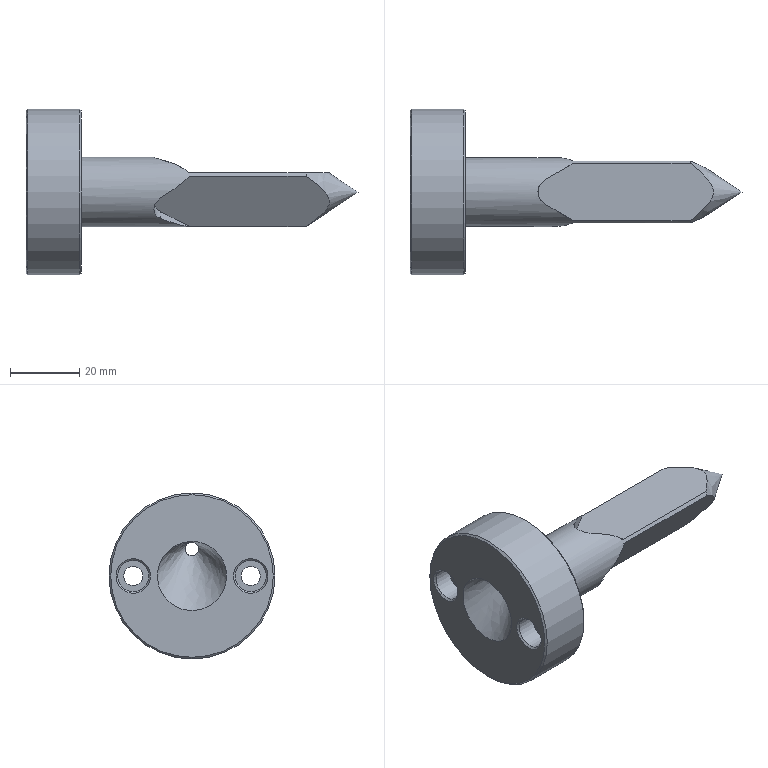NC program | NX | posted with a generic post | part box 96 x 48 x 48 mm
Lines 1 to 1795 of 1974, first 1661 of 1787 lines:
N10 G17 G21 G94 G90
(FLOOR_WALL , TOOL : D8)
N12 T08 M6
N14 G54
N16 G17 G0 G90 X-66.284 Y-8.048 S3500 M3
N18 G43 Z34.062 H8
N20 Z9.788
N22 G94 G1 X-69.517 Y-2.448 F1001.
N24 G3 X-70.21 Y-2.048 R0.8
N26 G1 X-95.937 F2200.
N28 Y2.048
N30 X-44.483
N32 X-41.035 Y0.
N34 X-44.482 Y-2.048
N36 X-70.21
N38 G3 X-70.903 Y-2.448 R0.8
N40 G1 X-74.136 Y-8.048
N42 G0 X-66.984 Y-8.881 Z9.576
N44 G1 X-70.218 Y-3.281 F1001.
N46 G3 X-70.91 Y-2.881 R0.8
N48 G1 X-95.937 F2200.
N50 Y2.881
N52 X-45.884
N54 X-41.035 Y0.
N56 X-45.883 Y-2.881
N58 X-70.91
N60 G3 X-71.603 Y-3.281 R0.8
N62 G1 X-74.836 Y-8.881
N64 G0 X-67.513 Y-9.509 Z9.364
N66 G1 X-70.746 Y-3.909 F1001.
N68 G3 X-71.439 Y-3.509 R0.8
N70 G1 X-95.937 F2200.
N72 Y3.509
N74 X-46.941
N76 X-41.035 Y0.
N78 X-46.941 Y-3.509
N80 X-71.439
N82 G3 X-72.132 Y-3.909 R0.8
N84 G1 X-75.365 Y-9.509
N86 G0 X-66.5 Y-10.029 Z9.152
N88 G1 X-69.733 Y-4.429 F1001.
N90 G3 X-70.426 Y-4.029 R0.8
N92 G1 X-95.937 F2200.
N94 Y4.029
N96 X-47.817
N98 X-41.035 Y0.
N100 X-47.817 Y-4.029
N102 X-70.426
N104 Y-0.029
N106 X-91.937
N108 Y0.029
N110 X-48.916
N112 X-48.866 Y0.
N114 X-48.915 Y-0.029
N116 X-70.426
N118 G3 X-71.119 Y-0.429 R0.8
N120 G1 Y-10.029
N122 G0 X-66.879 Y-10.48 Z8.94
N124 G1 X-70.113 Y-4.88 F1001.
N126 G3 X-70.805 Y-4.48 R0.8
N128 G1 X-95.937 F2200.
N130 Y4.48
N132 X-48.575
N134 X-41.035 Y0.
N136 X-48.575 Y-4.48
N138 X-70.805
N140 Y-0.48
N142 X-91.937
N144 Y0.48
N146 X-49.674
N148 X-48.866 Y0.
N150 X-49.674 Y-0.48
N152 X-70.805
N154 G3 X-71.498 Y-0.88 R0.8
N156 G1 Y-10.48
N158 G0 X-67.216 Y-10.88 Z8.729
N160 G1 X-70.449 Y-5.28 F1001.
N162 G3 X-71.142 Y-4.88 R0.8
N164 G1 X-95.92 F2200.
N166 X-95.937 Y-4.869
N168 Y4.869
N170 X-95.92 Y4.88
N172 X-49.249
N174 X-41.035 Y0.
N176 X-49.248 Y-4.88
N178 X-71.142
N180 Y-0.88
N182 X-91.937
N184 Y0.88
N186 X-50.347
N188 X-48.866 Y0.
N190 X-50.347 Y-0.88
N192 X-71.142
N194 G3 X-71.835 Y-1.28 R0.8
N196 G1 Y-10.88
N198 G0 X-67.52 Y-11.241 Z8.517
N200 G1 X-70.753 Y-5.641 F1001.
N202 G3 X-71.446 Y-5.241 R0.8
N204 G1 X-95.379 F2200.
N206 X-95.937 Y-4.869
N208 Y4.869
N210 X-95.379 Y5.241
N212 X-49.856
N214 X-41.035 Y0.
N216 X-49.856 Y-5.241
N218 X-71.446
N220 Y-1.241
N222 X-91.937
N224 Y1.241
N226 X-50.955
N228 X-48.866 Y0.
N230 X-50.955 Y-1.241
N232 X-71.446
N234 G3 X-72.139 Y-1.641 R0.8
N236 G1 Y-11.241
N238 G0 X-67.797 Y-11.571 Z8.305
N240 G1 X-71.031 Y-5.971 F1001.
N242 G3 X-71.723 Y-5.571 R0.8
N244 G1 X-94.884 F2200.
N246 X-95.937 Y-4.869
N248 Y4.869
N250 X-94.884 Y5.571
N252 X-50.411
N254 X-41.035 Y0.
N256 X-50.411 Y-5.571
N258 X-71.723
N260 Y-1.571
N262 X-91.937
N264 Y1.571
N266 X-51.51
N268 X-48.866 Y0.
N270 X-51.51 Y-1.571
N272 X-71.723
N274 G3 X-72.416 Y-1.971 R0.8
N276 G1 Y-11.571
N278 G0 X-68.053 Y-11.874 Z8.093
N280 G1 X-71.286 Y-6.274 F1001.
N282 G3 X-71.979 Y-5.874 R0.8
N284 G1 X-94.429 F2200.
N286 X-95.937 Y-4.869
N288 Y4.869
N290 X-94.429 Y5.874
N292 X-50.922
N294 X-41.035 Y0.
N296 X-50.922 Y-5.874
N298 X-71.979
N300 Y-1.874
N302 X-91.937
N304 Y1.874
N306 X-52.021
N308 X-48.866 Y0.
N310 X-52.021 Y-1.874
N312 X-71.979
N314 G3 X-72.672 Y-2.274 R0.8
N316 G1 Y-11.874
N318 G0 X-68.29 Y-12.156 Z7.881
N320 G1 X-71.523 Y-6.556 F1001.
N322 G3 X-72.216 Y-6.156 R0.8
N324 G1 X-94.007 F2200.
N326 X-95.937 Y-4.869
N328 Y4.869
N330 X-94.007 Y6.156
N332 X-51.396
N334 X-41.035 Y0.
N336 X-51.396 Y-6.156
N338 X-72.216
N340 Y-2.156
N342 X-91.937
N344 Y2.156
N346 X-52.494
N348 X-48.866 Y0.
N350 X-52.494 Y-2.156
N352 X-72.216
N354 G3 X-72.909 Y-2.556 R0.8
N356 G1 Y-12.156
N358 G0 X-68.51 Y-12.418 Z7.669
N360 G1 X-71.743 Y-6.818 F1001.
N362 G3 X-72.436 Y-6.418 R0.8
N364 G1 X-93.614 F2200.
N366 X-95.937 Y-4.869
N368 Y4.869
N370 X-93.614 Y6.418
N372 X-51.829
N374 X-41.035 Y0.
N376 X-51.829 Y-6.418
N378 X-72.436
N380 Y-2.418
N382 X-91.937
N384 Y2.418
N386 X-52.936
N388 X-48.866 Y0.
N390 X-52.935 Y-2.418
N392 X-72.436
N394 G3 X-73.129 Y-2.818 R0.8
N396 G1 Y-12.418
N398 G0 X-68.716 Y-12.663 Z7.457
N400 G1 X-71.95 Y-7.063 F1001.
N402 G3 X-72.642 Y-6.663 R0.8
N404 G1 X-93.246 F2200.
N406 X-95.937 Y-4.869
N408 Y4.869
N410 X-93.246 Y6.663
N412 X-51.762
N414 X-51.83 Y6.414
N416 X-41.035 Y0.
N418 X-51.83 Y-6.414
N420 X-51.762 Y-6.663
N422 X-72.642
N424 Y-2.663
N426 X-91.937
N428 Y2.663
N430 X-53.348
N432 X-48.866 Y0.
N434 X-53.348 Y-2.663
N436 X-72.642
N438 G3 X-73.335 Y-3.063 R0.8
N440 G1 Y-12.663
N442 G0 X-68.786 Y-12.892 Z7.245
N444 G1 X-72.02 Y-7.292 F1001.
N446 G3 X-72.712 Y-6.892 R0.8
N448 G1 X-92.901 F2200.
N450 X-95.937 Y-4.869
N452 Y4.869
N454 X-92.901 Y6.893
N456 X-51.699
N458 X-51.83 Y6.414
N460 X-41.035 Y0.
N462 X-51.83 Y-6.414
N464 X-51.699 Y-6.892
N466 X-72.712
N468 Y-2.892
N470 X-91.69
N472 X-91.937 Y-2.728
N474 Y2.728
N476 X-91.69 Y2.893
N478 X-53.735
N480 X-48.866 Y0.
N482 X-53.734 Y-2.892
N484 X-72.712
N486 G3 X-73.405 Y-3.292 R0.8
N488 G1 Y-12.892
N490 G0 X-68.799 Y-13.109 Z7.033
N492 G1 X-72.032 Y-7.509 F1001.
N494 G3 X-72.725 Y-7.109 R0.8
N496 G1 X-92.577 F2200.
N498 X-95.937 Y-4.869
N500 Y4.869
N502 X-92.577 Y7.109
N504 X-51.64
N506 X-51.83 Y6.414
N508 X-41.035 Y0.
N510 X-51.83 Y-6.414
N512 X-51.639 Y-7.109
N514 X-72.725
N516 Y-3.109
N518 X-91.366
N520 X-91.937 Y-2.728
N522 Y2.728
N524 X-91.366 Y3.109
N526 X-54.083
N528 G3 X-53.874 Y2.975 R4.
N530 G1 X-48.866 Y0.
N532 X-53.873 Y-2.975
N534 G3 X-54.083 Y-3.109 R4.
N536 G1 X-72.725
N538 G3 X-73.417 Y-3.509 R0.8
N540 G1 Y-13.109
N542 G0 X-68.782 Y-13.312 Z6.821
N544 G1 X-72.016 Y-7.712 F1001.
N546 G3 X-72.708 Y-7.312 R0.8
N548 G1 X-92.272 F2200.
N550 X-95.937 Y-4.869
N552 Y4.869
N554 X-92.272 Y7.312
N556 X-51.584
N558 X-51.83 Y6.414
N560 X-41.035 Y0.
N562 X-51.83 Y-6.414
N564 X-51.583 Y-7.312
N566 X-72.708
N568 Y-3.312
N570 X-91.061
N572 X-91.937 Y-2.728
N574 Y2.728
N576 X-91.061 Y3.312
N578 X-54.356
N580 G3 X-53.874 Y2.975 R4.
N582 G1 X-48.866 Y0.
N584 X-53.873 Y-2.975
N586 G3 X-54.356 Y-3.312 R4.
N588 G1 X-72.708
N590 G3 X-73.401 Y-3.712 R0.8
N592 G1 Y-13.312
N594 G0 X-68.748 Y-13.504 Z6.61
N596 G1 X-71.981 Y-7.904 F1001.
N598 G3 X-72.674 Y-7.504 R0.8
N600 G1 X-91.984 F2200.
N602 X-95.937 Y-4.869
N604 Y4.869
N606 X-91.983 Y7.504
N608 X-51.531
N610 X-51.83 Y6.414
N612 X-41.035 Y0.
N614 X-51.83 Y-6.414
N616 X-51.531 Y-7.504
N618 X-72.674
N620 Y-3.504
N622 X-90.773
N624 X-91.937 Y-2.728
N626 Y2.728
N628 X-90.772 Y3.504
N630 X-54.575
N632 G3 X-53.874 Y2.975 R4.
N634 G1 X-48.866 Y0.
N636 X-53.873 Y-2.975
N638 G3 X-54.575 Y-3.504 R4.
N640 G1 X-72.674
N642 G3 X-73.367 Y-3.904 R0.8
N644 G1 Y-13.504
N646 G0 X-68.262 Y-13.686 Z6.398
N648 G1 X-71.495 Y-8.086 F1001.
N650 G3 X-72.188 Y-7.686 R0.8
N652 G1 X-91.711 F2200.
N654 X-95.937 Y-4.869
N656 Y4.869
N658 X-91.711 Y7.686
N660 X-51.481
N662 X-51.83 Y6.414
N664 X-41.035 Y0.
N666 X-51.83 Y-6.414
N668 X-51.481 Y-7.686
N670 X-72.188
N672 Y-3.686
N674 X-90.5
N676 X-91.937 Y-2.728
N678 Y2.728
N680 X-90.5 Y3.686
N682 X-54.756
N684 G3 X-53.874 Y2.975 R4.
N686 G1 X-48.866 Y0.
N688 X-53.873 Y-2.975
N690 G3 X-54.755 Y-3.686 R4.
N692 G1 X-72.188
N694 Y-0.086
N696 X-88.337
N698 Y0.086
N700 X-56.039
N702 X-55.907 Y0.
N704 X-56.039 Y-0.086
N706 X-72.188
N708 G3 X-72.881 Y-0.486 R0.8
N710 G0 Z34.997
N712 X-72.382 Y-2.014 Z34.942
N714 X-71.882 Y-3.538 Z34.821
N716 X-71.383 Y-5.055 Z34.633
N718 X-70.883 Y-6.563 Z34.379
N720 X-70.384 Y-8.058 Z34.06
N722 X-69.884 Y-9.538 Z33.675
N724 X-69.385 Y-11. Z33.227
N726 X-68.885 Y-12.44 Z32.714
N728 X-68.386 Y-13.857 Z32.14
N730 Z6.186
N732 G1 X-71.619 Y-8.257 F1001.
N734 G3 X-72.312 Y-7.857 R0.8
N736 G1 X-91.454 F2200.
N738 X-95.937 Y-4.869
N740 Y4.869
N742 X-91.454 Y7.857
N744 X-51.434
N746 X-51.83 Y6.414
N748 X-41.035 Y0.
N750 X-51.83 Y-6.414
N752 X-51.434 Y-7.857
N754 X-72.312
N756 Y-3.857
N758 X-90.243
N760 X-91.937 Y-2.728
N762 Y2.728
N764 X-90.243 Y3.857
N766 X-54.907
N768 G3 X-53.874 Y2.975 R4.
N770 G1 X-48.866 Y0.
N772 X-53.873 Y-2.975
N774 G3 X-54.907 Y-3.857 R4.
N776 G1 X-72.312
N778 Y-0.257
N780 X-88.337
N782 Y0.257
N784 X-56.287
N786 G3 X-55.907 Y0. R7.6
N788 X-56.286 Y-0.257 R7.6
N790 G1 X-72.312
N792 G3 X-73.005 Y-0.657 R0.8
N794 G0 Z34.994
N796 X-72.489 Y-2.186 Z34.932
N798 X-71.973 Y-3.71 Z34.803
N800 X-71.457 Y-5.227 Z34.608
N802 X-70.941 Y-6.734 Z34.346
N804 X-70.425 Y-8.228 Z34.019
N806 X-69.909 Y-9.706 Z33.627
N808 X-69.393 Y-11.166 Z33.171
N810 X-68.877 Y-12.605 Z32.651
N812 X-68.362 Y-14.02 Z32.069
N814 Z5.974
N816 G1 X-71.595 Y-8.42 F1001.
N818 G3 X-72.288 Y-8.02 R0.8
N820 G1 X-91.211 F2200.
N822 X-95.937 Y-4.869
N824 Y4.869
N826 X-91.211 Y8.02
N828 X-51.389
N830 X-51.83 Y6.414
N832 X-41.035 Y0.
N834 X-51.83 Y-6.414
N836 X-51.389 Y-8.02
N838 X-72.288
N840 Y-4.02
N842 X-90.
N844 X-91.937 Y-2.728
N846 Y2.728
N848 X-89.999 Y4.02
N850 X-55.035
N852 G3 X-53.874 Y2.975 R4.
N854 G1 X-48.866 Y0.
N856 X-53.873 Y-2.975
N858 G3 X-55.034 Y-4.02 R4.
N860 G1 X-72.288
N862 Y-0.02
N864 X-87.937
N866 Y0.02
N868 X-56.638
N870 X-56.612 Y0.
N872 X-56.638 Y-0.02
N874 X-72.288
N876 G3 X-72.98 Y-0.42 R0.8
N878 G0 Z34.997
N880 X-72.478 Y-1.993 Z34.943
N882 X-71.976 Y-3.563 Z34.818
N884 X-71.474 Y-5.125 Z34.623
N886 X-70.971 Y-6.677 Z34.357
N888 X-70.469 Y-8.216 Z34.022
N890 X-69.967 Y-9.738 Z33.618
N892 X-69.465 Y-11.24 Z33.146
N894 X-68.963 Y-12.719 Z32.607
N896 X-68.46 Y-14.173 Z32.002
N898 Z5.762
N900 G1 X-71.694 Y-8.573 F1001.
N902 G3 X-72.386 Y-8.173 R0.8
N904 G1 X-90.98 F2200.
N906 X-95.937 Y-4.869
N908 Y4.869
N910 X-90.98 Y8.173
N912 X-51.347
N914 X-51.83 Y6.414
N916 X-41.035 Y0.
N918 X-51.83 Y-6.414
N920 X-51.347 Y-8.173
N922 X-72.386
N924 Y-4.173
N926 X-89.769
N928 X-91.937 Y-2.728
N930 Y2.728
N932 X-89.769 Y4.173
N934 X-55.144
N936 G3 X-53.874 Y2.975 R4.
N938 G1 X-48.866 Y0.
N940 X-53.873 Y-2.975
N942 G3 X-55.144 Y-4.173 R4.
N944 G1 X-72.386
N946 Y-0.173
N948 X-87.937
N950 Y0.173
N952 X-56.836
N954 G3 X-56.612 Y0. R8.
N956 X-56.836 Y-0.173 R8.
N958 G1 X-72.386
N960 G3 X-73.079 Y-0.573 R0.8
N962 G0 Z34.995
N964 X-72.576 Y-2.147 Z34.934
N966 X-72.072 Y-3.717 Z34.802
N968 X-71.569 Y-5.279 Z34.6
N970 X-71.066 Y-6.83 Z34.327
N972 X-70.562 Y-8.368 Z33.985
N974 X-70.059 Y-9.889 Z33.574
N976 X-69.555 Y-11.389 Z33.095
N978 X-69.052 Y-12.867 Z32.549
N980 X-68.548 Y-14.318 Z31.937
N982 Z5.55
N984 G1 X-71.782 Y-8.718 F1001.
N986 G3 X-72.474 Y-8.318 R0.8
N988 G1 X-90.762 F2200.
N990 X-95.937 Y-4.869
N992 Y4.869
N994 X-90.762 Y8.319
N996 X-51.307
N998 X-51.83 Y6.414
N1000 X-41.035 Y0.
N1002 X-51.83 Y-6.414
N1004 X-51.307 Y-8.318
N1006 X-72.474
N1008 Y-4.318
N1010 X-89.551
N1012 X-91.937 Y-2.728
N1014 Y2.728
N1016 X-89.551 Y4.319
N1018 X-55.238
N1020 G3 X-53.874 Y2.975 R4.
N1022 G1 X-48.866 Y0.
N1024 X-53.873 Y-2.975
N1026 G3 X-55.237 Y-4.318 R4.
N1028 G1 X-72.474
N1030 Y-0.318
N1032 X-87.937
N1034 Y0.319
N1036 X-57.012
N1038 G3 X-56.612 Y0. R8.
N1040 X-57.012 Y-0.318 R8.
N1042 G1 X-72.474
N1044 G3 X-73.167 Y-0.718 R0.8
N1046 G0 Z34.993
(FLOOR_WALL_COPY_1 , TOOL : D8)
N1048 X-66.284 Y33.523
N1050 Z-10.061
N1052 Y12.501 Z2.076
N1054 G1 X-69.517 Y9.701 Z-2.774 F1001.
N1056 X-69.689 Y9.591 Z-2.965
N1058 X-69.933 Y9.52 Z-3.087
N1060 X-70.21 Y9.501 Z-3.12
N1062 X-95.937 F2200.
N1064 Y7.453 Z-6.668
N1066 X-44.483
N1068 X-41.035 Y8.477 Z-4.894
N1070 X-44.482 Y9.501 Z-3.12
N1072 X-70.21
N1074 X-70.487 Y9.52 Z-3.087
N1076 X-70.73 Y9.591 Z-2.965
N1078 X-70.903 Y9.701 Z-2.774
N1080 X-74.136 Y12.501 Z2.076
N1082 G0 X-66.984 Y12.734 Z2.903
N1084 G1 X-70.218 Y9.934 Z-1.947 F1001.
N1086 X-70.39 Y9.823 Z-2.138
N1088 X-70.633 Y9.753 Z-2.26
N1090 X-70.91 Y9.734 Z-2.293
N1092 X-95.937 F2200.
N1094 Y6.853 Z-7.283
N1096 X-45.884
N1098 X-41.035 Y8.293 Z-4.788
N1100 X-45.883 Y9.734 Z-2.293
N1102 X-70.91
N1104 X-71.187 Y9.753 Z-2.26
N1106 X-71.431 Y9.823 Z-2.138
N1108 X-71.603 Y9.934 Z-1.947
N1110 X-74.836 Y12.734 Z2.903
N1112 G0 X-67.513 Y12.864 Z3.553
N1114 G1 X-70.746 Y10.064 Z-1.297 F1001.
N1116 X-70.918 Y9.954 Z-1.488
N1118 X-71.162 Y9.884 Z-1.61
N1120 X-71.439 Y9.864 Z-1.643
N1122 X-95.937 F2200.
N1124 Y6.355 Z-7.721
N1126 X-46.941
N1128 X-41.035 Y8.11 Z-4.682
N1130 X-46.941 Y9.864 Z-1.643
N1132 X-71.439
N1134 X-71.716 Y9.884 Z-1.61
N1136 X-71.96 Y9.954 Z-1.488
N1138 X-72.132 Y10.064 Z-1.297
N1140 X-75.365 Y12.864 Z3.553
N1142 G0 X-66.5 Y12.941 Z4.109
N1144 G1 X-69.733 Y10.141 Z-0.74 F1001.
N1146 X-69.906 Y10.031 Z-0.931
N1148 X-70.149 Y9.96 Z-1.053
N1150 X-70.426 Y9.941 Z-1.087
N1152 X-95.937 F2200.
N1154 Y5.912 Z-8.066
N1156 X-47.817
N1158 X-41.035 Y7.926 Z-4.576
N1160 X-47.817 Y9.941 Z-1.087
N1162 X-70.426
N1164 Y7.941 Z-4.551
N1166 X-91.937
N1168 Y7.912 Z-4.602
N1170 X-48.916
N1172 X-48.866 Y7.926 Z-4.576
N1174 X-48.915 Y7.941 Z-4.551
N1176 X-70.426
N1178 X-70.703 Y7.96 Z-4.517
N1180 X-70.947 Y8.031 Z-4.395
N1182 X-71.119 Y8.141 Z-4.204
N1184 Y12.941 Z4.109
N1186 G0 X-66.879 Y12.983 Z4.606
N1188 G1 X-70.113 Y10.183 Z-0.244 F1001.
N1190 X-70.285 Y10.072 Z-0.435
N1192 X-70.528 Y10.002 Z-0.557
N1194 X-70.805 Y9.983 Z-0.591
N1196 X-95.937 F2200.
N1198 Y5.503 Z-8.35
N1200 X-48.575
N1202 X-41.035 Y7.743 Z-4.47
N1204 X-48.575 Y9.983 Z-0.591
N1206 X-70.805
N1208 Y7.983 Z-4.055
N1210 X-91.937
N1212 Y7.503 Z-4.886
N1214 X-49.674
N1216 X-48.866 Y7.743 Z-4.47
N1218 X-49.674 Y7.983 Z-4.055
N1220 X-70.805
N1222 X-71.083 Y8.002 Z-4.021
N1224 X-71.326 Y8.072 Z-3.899
N1226 X-71.498 Y8.183 Z-3.708
N1228 Y12.983 Z4.606
N1230 G0 X-67.216 Y12.999 Z5.058
N1232 G1 X-70.449 Y10.199 Z0.208 F1001.
N1234 X-70.621 Y10.089 Z0.017
N1236 X-70.865 Y10.019 Z-0.105
N1238 X-71.142 Y9.999 Z-0.138
N1240 X-95.92 F2200.
N1242 X-95.937 Y9.994 Z-0.148
N1244 Y5.125 Z-8.581
N1246 X-95.92 Y5.119 Z-8.59
N1248 X-49.249
N1250 X-41.035 Y7.559 Z-4.364
N1252 X-49.248 Y9.999 Z-0.138
N1254 X-71.142
N1256 Y7.999 Z-3.602
N1258 X-91.937
N1260 Y7.119 Z-5.126
N1262 X-50.347
N1264 X-48.866 Y7.559 Z-4.364
N1266 X-50.347 Y7.999 Z-3.602
N1268 X-71.142
N1270 X-71.419 Y8.019 Z-3.569
N1272 X-71.663 Y8.089 Z-3.447
N1274 X-71.835 Y8.199 Z-3.256
N1276 Y12.999 Z5.058
N1278 G0 X-67.52 Y12.996 Z5.477
N1280 G1 X-70.753 Y10.196 Z0.627 F1001.
N1282 X-70.925 Y10.086 Z0.436
N1284 X-71.169 Y10.016 Z0.314
N1286 X-71.446 Y9.996 Z0.28
N1288 X-95.379 F2200.
N1290 X-95.937 Y9.81 Z-0.042
N1292 Y4.941 Z-8.475
N1294 X-95.379 Y4.755 Z-8.797
N1296 X-49.856
N1298 X-41.035 Y7.376 Z-4.258
N1300 X-49.856 Y9.996 Z0.28
N1302 X-71.446
N1304 Y7.996 Z-3.184
N1306 X-91.937
N1308 Y6.755 Z-5.333
N1310 X-50.955
N1312 X-48.866 Y7.376 Z-4.258
N1314 X-50.955 Y7.996 Z-3.184
N1316 X-71.446
N1318 X-71.723 Y8.016 Z-3.15
N1320 X-71.967 Y8.086 Z-3.028
N1322 X-72.139 Y8.196 Z-2.837
N1324 Y12.996 Z5.477
N1326 G0 X-67.797 Y12.977 Z5.868
N1328 G1 X-71.031 Y10.177 Z1.018 F1001.
N1330 X-71.203 Y10.067 Z0.827
N1332 X-71.446 Y9.997 Z0.706
N1334 X-71.723 Y9.977 Z0.672
N1336 X-94.884 F2200.
N1338 X-95.937 Y9.626 Z0.064
N1340 Y4.758 Z-8.369
N1342 X-94.884 Y4.407 Z-8.977
N1344 X-50.411
N1346 X-41.035 Y7.192 Z-4.152
N1348 X-50.411 Y9.977 Z0.672
N1350 X-71.723
N1352 Y7.977 Z-2.792
N1354 X-91.937
N1356 Y6.407 Z-5.513
N1358 X-51.51
N1360 X-48.866 Y7.192 Z-4.152
N1362 X-51.51 Y7.977 Z-2.792
N1364 X-71.723
N1366 X-72. Y7.997 Z-2.758
N1368 X-72.244 Y8.067 Z-2.637
N1370 X-72.416 Y8.177 Z-2.446
N1372 Y12.977 Z5.868
N1374 G0 X-68.053 Y12.946 Z6.237
N1376 G1 X-71.286 Y10.146 Z1.387 F1001.
N1378 X-71.458 Y10.036 Z1.196
N1380 X-71.702 Y9.965 Z1.074
N1382 X-71.979 Y9.946 Z1.041
N1384 X-94.429 F2200.
N1386 X-95.937 Y9.443 Z0.17
N1388 Y4.574 Z-8.263
N1390 X-94.429 Y4.072 Z-9.134
N1392 X-50.922
N1394 X-41.035 Y7.009 Z-4.046
N1396 X-50.922 Y9.946 Z1.041
N1398 X-71.979
N1400 Y7.946 Z-2.423
N1402 X-91.937
N1404 Y6.072 Z-5.67
N1406 X-52.021
N1408 X-48.866 Y7.009 Z-4.046
N1410 X-52.021 Y7.946 Z-2.423
N1412 X-71.979
N1414 X-72.256 Y7.965 Z-2.39
N1416 X-72.5 Y8.036 Z-2.268
N1418 X-72.672 Y8.146 Z-2.077
N1420 Y12.946 Z6.237
N1422 G0 X-68.29 Y12.903 Z6.587
N1424 G1 X-71.523 Y10.103 Z1.737 F1001.
N1426 X-71.695 Y9.993 Z1.546
N1428 X-71.939 Y9.922 Z1.424
N1430 X-72.216 Y9.903 Z1.39
N1432 X-94.007 F2200.
N1434 X-95.937 Y9.259 Z0.276
N1436 Y4.391 Z-8.157
N1438 X-94.007 Y3.747 Z-9.271
N1440 X-51.396
N1442 X-41.035 Y6.825 Z-3.94
N1444 X-51.396 Y9.903 Z1.39
N1446 X-72.216
N1448 Y7.903 Z-2.074
N1450 X-91.937
N1452 Y5.747 Z-5.807
N1454 X-52.494
N1456 X-48.866 Y6.825 Z-3.94
N1458 X-52.494 Y7.903 Z-2.074
N1460 X-72.216
N1462 X-72.493 Y7.922 Z-2.04
N1464 X-72.736 Y7.993 Z-1.918
N1466 X-72.909 Y8.103 Z-1.727
N1468 Y12.903 Z6.587
N1470 G0 X-68.51 Y12.85 Z6.92
N1472 G1 X-71.743 Y10.05 Z2.07 F1001.
N1474 X-71.916 Y9.94 Z1.879
N1476 X-72.159 Y9.87 Z1.757
N1478 X-72.436 Y9.85 Z1.723
N1480 X-93.614 F2200.
N1482 X-95.937 Y9.076 Z0.382
N1484 Y4.207 Z-8.051
N1486 X-93.614 Y3.433 Z-9.392
N1488 X-51.829
N1490 X-41.035 Y6.642 Z-3.834
N1492 X-51.829 Y9.85 Z1.723
N1494 X-72.436
N1496 Y7.85 Z-1.741
N1498 X-91.937
N1500 Y5.433 Z-5.928
N1502 X-52.936
N1504 X-48.866 Y6.642 Z-3.834
N1506 X-52.935 Y7.85 Z-1.741
N1508 X-72.436
N1510 X-72.713 Y7.87 Z-1.707
N1512 X-72.957 Y7.94 Z-1.585
N1514 X-73.129 Y8.05 Z-1.394
N1516 Y12.85 Z6.92
N1518 G0 X-68.716 Y12.789 Z7.238
N1520 G1 X-71.95 Y9.989 Z2.388 F1001.
N1522 X-72.122 Y9.879 Z2.197
N1524 X-72.365 Y9.809 Z2.075
N1526 X-72.642 Y9.789 Z2.042
N1528 X-93.246 F2200.
N1530 X-95.937 Y8.892 Z0.488
N1532 Y4.024 Z-7.945
N1534 X-93.246 Y3.127 Z-9.499
N1536 X-51.762
N1538 X-51.83 Y3.251 Z-9.283
N1540 X-41.035 Y6.458 Z-3.728
N1542 X-51.83 Y9.665 Z1.826
N1544 X-51.762 Y9.789 Z2.042
N1546 X-72.642
N1548 Y7.789 Z-1.423
N1550 X-91.937
N1552 Y5.127 Z-6.035
N1554 X-53.348
N1556 X-48.866 Y6.458 Z-3.728
N1558 X-53.348 Y7.789 Z-1.423
N1560 X-72.642
N1562 X-72.919 Y7.809 Z-1.389
N1564 X-73.163 Y7.879 Z-1.267
N1566 X-73.335 Y7.989 Z-1.076
N1568 Y12.789 Z7.238
N1570 G0 X-68.786 Y12.721 Z7.543
N1572 G1 X-72.02 Y9.921 Z2.693 F1001.
N1574 X-72.192 Y9.811 Z2.502
N1576 X-72.435 Y9.74 Z2.38
N1578 X-72.712 Y9.721 Z2.347
N1580 X-92.901 F2200.
N1582 X-95.937 Y8.709 Z0.594
N1584 Y3.84 Z-7.839
N1586 X-92.901 Y2.828 Z-9.592
N1588 X-51.699
N1590 X-51.83 Y3.068 Z-9.177
N1592 X-41.035 Y6.275 Z-3.623
N1594 X-51.83 Y9.482 Z1.932
N1596 X-51.699 Y9.721 Z2.347
N1598 X-72.712
N1600 Y7.721 Z-1.118
N1602 X-91.69
N1604 X-91.937 Y7.639 Z-1.26
N1606 Y4.911 Z-5.985
N1608 X-91.69 Y4.828 Z-6.128
N1610 X-53.735
N1612 X-48.866 Y6.275 Z-3.623
N1614 X-53.734 Y7.721 Z-1.118
N1616 X-72.712
N1618 X-72.989 Y7.74 Z-1.084
N1620 X-73.233 Y7.811 Z-0.962
N1622 X-73.405 Y7.921 Z-0.771
N1624 Y12.721 Z7.543
N1626 G0 X-68.799 Y12.645 Z7.836
N1628 G1 X-72.032 Y9.845 Z2.986 F1001.
N1630 X-72.204 Y9.735 Z2.795
N1632 X-72.448 Y9.665 Z2.673
N1634 X-72.725 Y9.645 Z2.64
N1636 X-92.577 F2200.
N1638 X-95.937 Y8.525 Z0.7
N1640 Y3.657 Z-7.733
N1642 X-92.577 Y2.537 Z-9.673
N1644 X-51.64
N1646 X-51.83 Y2.884 Z-9.071
N1648 X-41.035 Y6.091 Z-3.517
N1650 X-51.83 Y9.298 Z2.038
N1652 X-51.639 Y9.645 Z2.64
N1654 X-72.725
N1656 Y7.645 Z-0.824
N1658 X-91.366
N1660 X-91.937 Y7.455 Z-1.154
N1662 Y4.727 Z-5.879
N1664 X-91.366 Y4.537 Z-6.209
N1666 X-54.083
N1668 X-53.874 Y4.604 Z-6.093
N1670 X-48.866 Y6.091 Z-3.517
N1672 X-53.873 Y7.579 Z-0.94
N1674 X-54.083 Y7.645 Z-0.824
N1676 X-72.725
N1678 X-73.002 Y7.665 Z-0.791
N1680 X-73.245 Y7.735 Z-0.669
N1682 X-73.417 Y7.845 Z-0.478
N1684 Y12.645 Z7.836
N1686 G0 X-68.782 Y12.564 Z8.118
N1688 G1 X-72.016 Y9.764 Z3.268 F1001.
N1690 X-72.188 Y9.653 Z3.077
N1692 X-72.431 Y9.583 Z2.956
N1694 X-72.708 Y9.564 Z2.922
N1696 X-92.272 F2200.
N1698 X-95.937 Y8.342 Z0.806
N1700 Y3.473 Z-7.627
N1702 X-92.272 Y2.251 Z-9.743
N1704 X-51.584
N1706 X-51.83 Y2.701 Z-8.965
N1708 X-41.035 Y5.908 Z-3.411
N1710 X-51.83 Y9.114 Z2.144
N1712 X-51.583 Y9.564 Z2.922
N1714 X-72.708
N1716 Y7.564 Z-0.542
N1718 X-91.061
N1720 X-91.937 Y7.272 Z-1.048
N1722 Y4.544 Z-5.773
N1724 X-91.061 Y4.251 Z-6.279
N1726 X-54.356
N1728 X-54.207 Y4.316 Z-6.168
N1730 X-54.045 Y4.372 Z-6.07
N1732 X-53.874 Y4.42 Z-5.987
N1734 X-48.866 Y5.908 Z-3.411
N1736 X-53.873 Y7.395 Z-0.834
N1738 X-54.045 Y7.443 Z-0.751
N1740 X-54.207 Y7.5 Z-0.653
N1742 X-54.356 Y7.564 Z-0.542
N1744 X-72.708
N1746 X-72.985 Y7.583 Z-0.509
N1748 X-73.229 Y7.653 Z-0.387
N1750 X-73.401 Y7.764 Z-0.196
N1752 Y12.564 Z8.118
N1754 G0 X-68.748 Y12.476 Z8.39
N1756 G1 X-71.981 Y9.676 Z3.541 F1001.
N1758 X-72.153 Y9.566 Z3.35
N1760 X-72.397 Y9.496 Z3.228
N1762 X-72.674 Y9.476 Z3.194
N1764 X-91.984 F2200.
N1766 X-95.937 Y8.158 Z0.912
N1768 Y3.29 Z-7.521
N1770 X-91.983 Y1.972 Z-9.804
N1772 X-51.531
N1774 X-51.83 Y2.517 Z-8.859
N1776 X-41.035 Y5.724 Z-3.305
N1778 X-51.83 Y8.931 Z2.25
N1780 X-51.531 Y9.476 Z3.194
N1782 X-72.674
N1784 Y7.476 Z-0.27
N1786 X-90.773
N1788 X-91.937 Y7.088 Z-0.942
N1790 Y4.36 Z-5.667
N1792 X-90.772 Y3.972 Z-6.34
N1794 X-54.575
N1796 X-54.361 Y4.073 Z-6.165
N1798 X-54.126 Y4.161 Z-6.012
N1800 X-53.874 Y4.237 Z-5.881
N1802 X-48.866 Y5.724 Z-3.305
N1804 X-53.873 Y7.212 Z-0.728
N1806 X-54.126 Y7.287 Z-0.598
N1808 X-54.361 Y7.376 Z-0.444
N1810 X-54.575 Y7.476 Z-0.27
N1812 X-72.674
N1814 X-72.951 Y7.496 Z-0.236
N1816 X-73.194 Y7.566 Z-0.114
N1818 X-73.367 Y7.676 Z0.076
N1820 Y12.476 Z8.39
N1822 G0 X-68.262 Y12.383 Z8.653
N1824 G1 X-71.495 Y9.583 Z3.804 F1001.
N1826 X-71.668 Y9.473 Z3.613
N1828 X-71.911 Y9.403 Z3.491
N1830 X-72.188 Y9.383 Z3.457
N1832 X-91.711 F2200.
N1834 X-95.937 Y7.975 Z1.018
N1836 Y3.106 Z-7.415
N1838 X-91.711 Y1.698 Z-9.855
N1840 X-51.481
N1842 X-51.83 Y2.334 Z-8.753
N1844 X-41.035 Y5.541 Z-3.199
N1846 X-51.83 Y8.747 Z2.356
N1848 X-51.481 Y9.383 Z3.457
N1850 X-72.188
N1852 Y7.383 Z-0.007
N1854 X-90.5
N1856 X-91.937 Y6.905 Z-0.836
N1858 Y4.177 Z-5.561
N1860 X-90.5 Y3.698 Z-6.391
N1862 X-54.756
N1864 X-54.491 Y3.834 Z-6.155
N1866 X-54.196 Y3.953 Z-5.949
N1868 X-53.874 Y4.053 Z-5.775
N1870 X-48.866 Y5.541 Z-3.199
N1872 X-53.873 Y7.028 Z-0.622
N1874 X-54.195 Y7.128 Z-0.449
N1876 X-54.491 Y7.247 Z-0.242
N1878 X-54.755 Y7.383 Z-0.007
N1880 X-72.188
N1882 Y5.583 Z-3.125
N1884 X-88.337
N1886 Y5.498 Z-3.273
N1888 X-56.039
N1890 X-55.907 Y5.541 Z-3.199
N1892 X-56.039 Y5.583 Z-3.125
N1894 X-72.188
N1896 X-72.465 Y5.603 Z-3.091
N1898 X-72.709 Y5.673 Z-2.969
N1900 X-72.881 Y5.783 Z-2.778
N1902 G0 Y30.551 Z-17.078
N1904 X-72.382 Y31.268 Z-15.727
N1906 X-71.882 Y31.925 Z-14.346
N1908 X-71.383 Y32.521 Z-12.938
N1910 X-70.883 Y33.055 Z-11.506
N1912 X-70.384 Y33.526 Z-10.051
N1914 X-69.884 Y33.933 Z-8.577
N1916 X-69.385 Y34.275 Z-7.087
N1918 X-68.885 Y34.552 Z-5.584
N1920 X-68.386 Y34.763 Z-4.069
N1922 Y12.286 Z8.908
N1924 G1 X-71.619 Y9.486 Z4.058 F1001.
N1926 X-71.791 Y9.375 Z3.867
N1928 X-72.035 Y9.305 Z3.745
N1930 X-72.312 Y9.286 Z3.712
N1932 X-91.454 F2200.
N1934 X-95.937 Y7.791 Z1.124
N1936 Y2.923 Z-7.309
N1938 X-91.454 Y1.428 Z-9.897
N1940 X-51.434
N1942 X-51.83 Y2.15 Z-8.647
N1944 X-41.035 Y5.357 Z-3.093
N1946 X-51.83 Y8.564 Z2.462
N1948 X-51.434 Y9.286 Z3.712
N1950 X-72.312
N1952 Y7.286 Z0.248
N1954 X-90.243
N1956 X-91.937 Y6.721 Z-0.73
N1958 Y3.993 Z-5.455
N1960 X-90.243 Y3.428 Z-6.433
N1962 X-54.907
N1964 X-54.604 Y3.598 Z-6.139
N1966 X-54.257 Y3.746 Z-5.882
N1968 X-53.874 Y3.87 Z-5.669
N1970 X-48.866 Y5.357 Z-3.093
N1972 X-53.873 Y6.845 Z-0.516
N1974 X-54.256 Y6.968 Z-0.303
N1976 X-54.603 Y7.116 Z-0.047
N1978 X-54.907 Y7.286 Z0.248
N1980 X-72.312
N1982 Y5.486 Z-2.87
N1984 X-88.337
N1986 Y5.228 Z-3.316
N1988 X-56.287
N1990 X-56.105 Y5.298 Z-3.195
N1992 X-55.907 Y5.357 Z-3.093
N1994 X-56.104 Y5.416 Z-2.991
N1996 X-56.286 Y5.486 Z-2.87
N1998 X-72.312
N2000 X-72.589 Y5.505 Z-2.836
N2002 X-72.832 Y5.575 Z-2.715
N2004 X-73.005 Y5.686 Z-2.524
N2006 G0 Y30.634 Z-16.928
N2008 X-72.489 Y31.345 Z-15.573
N2010 X-71.973 Y31.995 Z-14.189
N2012 X-71.457 Y32.584 Z-12.777
N2014 X-70.941 Y33.112 Z-11.341
N2016 X-70.425 Y33.575 Z-9.884
N2018 X-69.909 Y33.975 Z-8.408
N2020 X-69.393 Y34.31 Z-6.915
N2022 X-68.877 Y34.58 Z-5.409
N2024 X-68.362 Y34.783 Z-3.893
N2026 Y12.183 Z9.154
N2028 G1 X-71.595 Y9.383 Z4.305 F1001.
N2030 X-71.767 Y9.273 Z4.114
N2032 X-72.01 Y9.203 Z3.992
N2034 X-72.288 Y9.183 Z3.958
N2036 X-91.211 F2200.
N2038 X-95.937 Y7.608 Z1.229
N2040 Y2.739 Z-7.203
N2042 X-91.211 Y1.164 Z-9.932
N2044 X-51.389
N2046 X-51.83 Y1.967 Z-8.541
N2048 X-41.035 Y5.174 Z-2.987
N2050 X-51.83 Y8.38 Z2.568
N2052 X-51.389 Y9.183 Z3.958
N2054 X-72.288
N2056 Y7.183 Z0.494
N2058 X-90.
N2060 X-91.937 Y6.537 Z-0.624
N2062 Y3.81 Z-5.349
N2064 X-89.999 Y3.164 Z-6.468
N2066 X-55.035
N2068 X-54.702 Y3.366 Z-6.117
N2070 X-54.311 Y3.542 Z-5.813
N2072 X-53.874 Y3.686 Z-5.563
N2074 X-48.866 Y5.174 Z-2.987
N2076 X-53.873 Y6.661 Z-0.411
N2078 X-54.311 Y6.805 Z-0.161
N2080 X-54.701 Y6.981 Z0.143
N2082 X-55.034 Y7.183 Z0.494
N2084 X-72.288
N2086 Y5.183 Z-2.97
N2088 X-87.937
N2090 Y5.164 Z-3.004
N2092 X-56.638
N2094 X-56.612 Y5.174 Z-2.987
N2096 X-56.638 Y5.183 Z-2.97
N2098 X-72.288
N2100 X-72.565 Y5.203 Z-2.936
N2102 X-72.808 Y5.273 Z-2.814
N2104 X-72.98 Y5.383 Z-2.624
N2106 G0 Y30.519 Z-17.135
N2108 X-72.478 Y31.258 Z-15.745
N2110 X-71.976 Y31.935 Z-14.324
N2112 X-71.474 Y32.547 Z-12.873
N2114 X-70.971 Y33.093 Z-11.396
N2116 X-70.469 Y33.572 Z-9.896
N2118 X-69.967 Y33.983 Z-8.376
N2120 X-69.465 Y34.325 Z-6.839
N2122 X-68.963 Y34.598 Z-5.288
N2124 X-68.46 Y34.801 Z-3.727
N2126 Y12.077 Z9.393
N2128 G1 X-71.694 Y9.277 Z4.544 F1001.
N2130 X-71.866 Y9.166 Z4.353
N2132 X-72.109 Y9.096 Z4.231
N2134 X-72.386 Y9.077 Z4.197
N2136 X-90.98 F2200.
N2138 X-95.937 Y7.424 Z1.335
N2140 Y2.556 Z-7.097
N2142 X-90.98 Y0.903 Z-9.959
N2144 X-51.347
N2146 X-51.83 Y1.783 Z-8.435
N2148 X-41.035 Y4.99 Z-2.881
N2150 X-51.83 Y8.197 Z2.674
N2152 X-51.347 Y9.077 Z4.197
N2154 X-72.386
N2156 Y7.077 Z0.733
N2158 X-89.769
N2160 X-91.937 Y6.354 Z-0.519
N2162 Y3.626 Z-5.243
N2164 X-89.769 Y2.903 Z-6.495
N2166 X-55.144
N2168 X-54.788 Y3.137 Z-6.091
N2170 X-54.361 Y3.339 Z-5.741
N2172 X-53.874 Y3.503 Z-5.457
N2174 X-48.866 Y4.99 Z-2.881
N2176 X-53.873 Y6.478 Z-0.305
N2178 X-54.36 Y6.641 Z-0.021
N2180 X-54.788 Y6.843 Z0.329
N2182 X-55.144 Y7.077 Z0.733
N2184 X-72.386
N2186 Y5.077 Z-2.731
N2188 X-87.937
N2190 Y4.903 Z-3.031
N2192 X-56.836
N2194 X-56.612 Y4.99 Z-2.881
N2196 X-56.836 Y5.077 Z-2.731
N2198 X-72.386
N2200 X-72.663 Y5.096 Z-2.697
N2202 X-72.907 Y5.166 Z-2.576
N2204 X-73.079 Y5.277 Z-2.385
N2206 G0 Y30.593 Z-17.001
N2208 X-72.576 Y31.327 Z-15.608
N2210 X-72.072 Y31.998 Z-14.182
N2212 X-71.569 Y32.604 Z-12.728
N2214 X-71.066 Y33.143 Z-11.248
N2216 X-70.562 Y33.616 Z-9.745
N2218 X-70.059 Y34.02 Z-8.223
N2220 X-69.555 Y34.356 Z-6.684
N2222 X-69.052 Y34.622 Z-5.131
N2224 X-68.548 Y34.818 Z-3.568
N2226 Y11.966 Z9.625
N2228 G1 X-71.782 Y9.166 Z4.775 F1001.
N2230 X-71.954 Y9.056 Z4.584
N2232 X-72.197 Y8.985 Z4.463
N2234 X-72.474 Y8.966 Z4.429
N2236 X-90.762 F2200.
N2238 X-95.937 Y7.241 Z1.441
N2240 Y2.372 Z-6.991
N2242 X-90.762 Y0.647 Z-9.979
N2244 X-51.307
N2246 X-51.83 Y1.6 Z-8.33
N2248 X-41.035 Y4.807 Z-2.775
N2250 X-51.83 Y8.013 Z2.78
N2252 X-51.307 Y8.966 Z4.429
N2254 X-72.474
N2256 Y6.966 Z0.965
N2258 X-89.551
N2260 X-91.937 Y6.17 Z-0.413
N2262 Y3.443 Z-5.137
N2264 X-89.551 Y2.647 Z-6.515
N2266 X-55.238
N2268 X-54.865 Y2.91 Z-6.059
N2270 X-54.405 Y3.137 Z-5.667
N2272 X-53.874 Y3.319 Z-5.351
N2274 X-48.866 Y4.807 Z-2.775
N2276 X-53.873 Y6.294 Z-0.199
N2278 X-54.405 Y6.476 Z0.117
N2280 X-54.865 Y6.703 Z0.509
N2282 X-55.237 Y6.966 Z0.965
N2284 X-72.474
N2286 Y4.966 Z-2.499
N2288 X-87.937
N2290 Y4.647 Z-3.051
N2292 X-57.012
N2294 X-56.821 Y4.732 Z-2.903
N2296 X-56.612 Y4.807 Z-2.775
N2298 X-56.82 Y4.881 Z-2.647
N2300 X-57.012 Y4.966 Z-2.499
N2302 X-72.474
N2304 X-72.751 Y4.985 Z-2.466
N2306 X-72.995 Y5.056 Z-2.344
N2308 X-73.167 Y5.166 Z-2.153
N2310 G0 Y30.664 Z-16.874
(FLOOR_WALL_COPY_2 , TOOL : D8)
N2312 X-66.284 Y-25.474
N2314 Z-24.001
N2316 Y-4.452 Z-11.864
N2318 G1 X-69.517 Y-7.252 Z-7.014 F1001.
N2320 X-69.689 Y-7.363 Z-6.823
N2322 X-69.933 Y-7.433 Z-6.701
N2324 X-70.21 Y-7.452 Z-6.668
N2326 X-95.937 F2200.
N2328 Y-9.501 Z-3.12
N2330 X-44.483
N2332 X-41.035 Y-8.477 Z-4.894
N2334 X-44.482 Y-7.452 Z-6.668
N2336 X-70.21
N2338 X-70.487 Y-7.433 Z-6.701
N2340 X-70.73 Y-7.363 Z-6.823
N2342 X-70.903 Y-7.252 Z-7.014
N2344 X-74.136 Y-4.452 Z-11.864
N2346 G0 X-66.984 Y-3.853 Z-12.479
N2348 G1 X-70.218 Y-6.653 Z-7.629 F1001.
N2350 X-70.39 Y-6.763 Z-7.438
N2352 X-70.633 Y-6.833 Z-7.316
N2354 X-70.91 Y-6.853 Z-7.283
N2356 X-95.937 F2200.
N2358 Y-9.733 Z-2.293
N2360 X-45.884
N2362 X-41.035 Y-8.293 Z-4.788
N2364 X-45.883 Y-6.853 Z-7.283
N2366 X-70.91
N2368 X-71.187 Y-6.833 Z-7.316
N2370 X-71.431 Y-6.763 Z-7.438
N2372 X-71.603 Y-6.653 Z-7.629
N2374 X-74.836 Y-3.853 Z-12.479
N2376 G0 X-67.513 Y-3.355 Z-12.917
N2378 G1 X-70.746 Y-6.155 Z-8.067 F1001.
N2380 X-70.918 Y-6.265 Z-7.876
N2382 X-71.162 Y-6.336 Z-7.754
N2384 X-71.439 Y-6.355 Z-7.721
N2386 X-95.937 F2200.
N2388 Y-9.864 Z-1.643
N2390 X-46.941
N2392 X-41.035 Y-8.11 Z-4.682
N2394 X-46.941 Y-6.355 Z-7.721
N2396 X-71.439
N2398 X-71.716 Y-6.336 Z-7.754
N2400 X-71.96 Y-6.265 Z-7.876
N2402 X-72.132 Y-6.155 Z-8.067
N2404 X-75.365 Y-3.355 Z-12.917
N2406 G0 X-66.5 Y-2.911 Z-13.262
N2408 G1 X-69.733 Y-5.711 Z-8.412 F1001.
N2410 X-69.906 Y-5.822 Z-8.221
N2412 X-70.149 Y-5.892 Z-8.099
N2414 X-70.426 Y-5.911 Z-8.066
N2416 X-95.937 F2200.
N2418 Y-9.941 Z-1.087
N2420 X-47.817
N2422 X-41.035 Y-7.926 Z-4.576
N2424 X-47.817 Y-5.911 Z-8.066
N2426 X-70.426
N2428 Y-7.911 Z-4.602
N2430 X-91.937
N2432 Y-7.941 Z-4.551
N2434 X-48.916
N2436 X-48.866 Y-7.926 Z-4.576
N2438 X-48.915 Y-7.911 Z-4.602
N2440 X-70.426
N2442 X-70.703 Y-7.892 Z-4.635
N2444 X-70.947 Y-7.822 Z-4.757
N2446 X-71.119 Y-7.711 Z-4.948
N2448 Y-2.911 Z-13.262
N2450 G0 X-66.879 Y-2.503 Z-13.546
N2452 G1 X-70.113 Y-5.303 Z-8.696 F1001.
N2454 X-70.285 Y-5.413 Z-8.505
N2456 X-70.528 Y-5.483 Z-8.384
N2458 X-70.805 Y-5.503 Z-8.35
N2460 X-95.937 F2200.
N2462 Y-9.982 Z-0.591
N2464 X-48.575
N2466 X-41.035 Y-7.742 Z-4.47
N2468 X-48.575 Y-5.503 Z-8.35
N2470 X-70.805
N2472 Y-7.503 Z-4.886
N2474 X-91.937
N2476 Y-7.982 Z-4.055
N2478 X-49.674
N2480 X-48.866 Y-7.742 Z-4.47
N2482 X-49.674 Y-7.503 Z-4.886
N2484 X-70.805
N2486 X-71.083 Y-7.483 Z-4.919
N2488 X-71.326 Y-7.413 Z-5.041
N2490 X-71.498 Y-7.303 Z-5.232
N2492 Y-2.503 Z-13.546
N2494 G0 X-67.216 Y-2.119 Z-13.787
N2496 G1 X-70.449 Y-4.919 Z-8.937 F1001.
N2498 X-70.621 Y-5.029 Z-8.746
N2500 X-70.865 Y-5.1 Z-8.624
N2502 X-71.142 Y-5.119 Z-8.59
N2504 X-95.92 F2200.
N2506 X-95.937 Y-5.125 Z-8.581
N2508 Y-9.993 Z-0.148
N2510 X-95.92 Y-9.999 Z-0.138
N2512 X-49.249
N2514 X-41.035 Y-7.559 Z-4.364
N2516 X-49.248 Y-5.119 Z-8.59
N2518 X-71.142
N2520 Y-7.119 Z-5.126
N2522 X-91.937
N2524 Y-7.999 Z-3.602
N2526 X-50.347
N2528 X-48.866 Y-7.559 Z-4.364
N2530 X-50.347 Y-7.119 Z-5.126
N2532 X-71.142
N2534 X-71.419 Y-7.1 Z-5.16
N2536 X-71.663 Y-7.029 Z-5.282
N2538 X-71.835 Y-6.919 Z-5.473
N2540 Y-2.119 Z-13.787
N2542 G0 X-67.52 Y-1.755 Z-13.993
N2544 G1 X-70.753 Y-4.555 Z-9.144 F1001.
N2546 X-70.925 Y-4.665 Z-8.953
N2548 X-71.169 Y-4.736 Z-8.831
N2550 X-71.446 Y-4.755 Z-8.797
N2552 X-95.379 F2200.
N2554 X-95.937 Y-4.941 Z-8.475
N2556 Y-9.81 Z-0.042
N2558 X-95.379 Y-9.996 Z0.28
N2560 X-49.856
N2562 X-41.035 Y-7.375 Z-4.258
N2564 X-49.856 Y-4.755 Z-8.797
N2566 X-71.446
N2568 Y-6.755 Z-5.333
N2570 X-91.937
N2572 Y-7.996 Z-3.184
N2574 X-50.955
N2576 X-48.866 Y-7.375 Z-4.258
N2578 X-50.955 Y-6.755 Z-5.333
N2580 X-71.446
N2582 X-71.723 Y-6.736 Z-5.367
N2584 X-71.967 Y-6.665 Z-5.488
N2586 X-72.139 Y-6.555 Z-5.679
N2588 Y-1.755 Z-13.993
N2590 G0 X-67.797 Y-1.407 Z-14.173
N2592 G1 X-71.031 Y-4.207 Z-9.323 F1001.
N2594 X-71.203 Y-4.317 Z-9.132
N2596 X-71.446 Y-4.387 Z-9.01
N2598 X-71.723 Y-4.407 Z-8.977
N2600 X-94.884 F2200.
N2602 X-95.937 Y-4.758 Z-8.369
N2604 Y-9.626 Z0.064
N2606 X-94.884 Y-9.977 Z0.672
N2608 X-50.411
N2610 X-41.035 Y-7.192 Z-4.152
N2612 X-50.411 Y-4.407 Z-8.977
N2614 X-71.723
N2616 Y-6.407 Z-5.513
N2618 X-91.937
N2620 Y-7.977 Z-2.792
N2622 X-51.51
N2624 X-48.866 Y-7.192 Z-4.152
N2626 X-51.51 Y-6.407 Z-5.513
N2628 X-71.723
N2630 X-72. Y-6.387 Z-5.546
N2632 X-72.244 Y-6.317 Z-5.668
N2634 X-72.416 Y-6.207 Z-5.859
N2636 Y-1.407 Z-14.173
N2638 G0 X-68.053 Y-1.071 Z-14.33
N2640 G1 X-71.286 Y-3.871 Z-9.48 F1001.
N2642 X-71.458 Y-3.982 Z-9.289
N2644 X-71.702 Y-4.052 Z-9.167
N2646 X-71.979 Y-4.071 Z-9.134
N2648 X-94.429 F2200.
N2650 X-95.937 Y-4.574 Z-8.263
N2652 Y-9.443 Z0.17
N2654 X-94.429 Y-9.946 Z1.041
N2656 X-50.922
N2658 X-41.035 Y-7.008 Z-4.046
N2660 X-50.922 Y-4.071 Z-9.134
N2662 X-71.979
N2664 Y-6.071 Z-5.67
N2666 X-91.937
N2668 Y-7.946 Z-2.423
N2670 X-52.021
N2672 X-48.866 Y-7.008 Z-4.046
N2674 X-52.021 Y-6.071 Z-5.67
N2676 X-71.979
N2678 X-72.256 Y-6.052 Z-5.703
N2680 X-72.5 Y-5.982 Z-5.825
N2682 X-72.672 Y-5.871 Z-6.016
N2684 Y-1.071 Z-14.33
N2686 G0 X-68.29 Y-0.747 Z-14.468
N2688 G1 X-71.523 Y-3.547 Z-9.618 F1001.
N2690 X-71.695 Y-3.657 Z-9.427
N2692 X-71.939 Y-3.728 Z-9.305
N2694 X-72.216 Y-3.747 Z-9.271
N2696 X-94.007 F2200.
N2698 X-95.937 Y-4.391 Z-8.157
N2700 Y-9.259 Z0.276
N2702 X-94.007 Y-9.903 Z1.39
N2704 X-51.396
N2706 X-41.035 Y-6.825 Z-3.941
N2708 X-51.396 Y-3.747 Z-9.271
N2710 X-72.216
N2712 Y-5.747 Z-5.807
N2714 X-91.937
N2716 Y-7.903 Z-2.074
N2718 X-52.494
N2720 X-48.866 Y-6.825 Z-3.941
N2722 X-52.494 Y-5.747 Z-5.807
N2724 X-72.216
N2726 X-72.493 Y-5.728 Z-5.841
N2728 X-72.736 Y-5.657 Z-5.963
N2730 X-72.909 Y-5.547 Z-6.154
N2732 Y-0.747 Z-14.468
N2734 G0 X-68.51 Y-0.433 Z-14.589
N2736 G1 X-71.743 Y-3.233 Z-9.739 F1001.
N2738 X-71.916 Y-3.343 Z-9.548
N2740 X-72.159 Y-3.413 Z-9.426
N2742 X-72.436 Y-3.433 Z-9.392
N2744 X-93.614 F2200.
N2746 X-95.937 Y-4.207 Z-8.051
N2748 Y-9.076 Z0.382
N2750 X-93.614 Y-9.85 Z1.723
N2752 X-51.829
N2754 X-41.035 Y-6.641 Z-3.835
N2756 X-51.829 Y-3.433 Z-9.392
N2758 X-72.436
N2760 Y-5.433 Z-5.928
N2762 X-91.937
N2764 Y-7.85 Z-1.741
N2766 X-52.936
N2768 X-48.866 Y-6.641 Z-3.835
N2770 X-52.935 Y-5.433 Z-5.928
N2772 X-72.436
N2774 X-72.713 Y-5.413 Z-5.962
N2776 X-72.957 Y-5.343 Z-6.084
N2778 X-73.129 Y-5.233 Z-6.275
N2780 Y-0.433 Z-14.589
N2782 G0 X-68.716 Y-0.127 Z-14.695
N2784 G1 X-71.95 Y-2.927 Z-9.845 F1001.
N2786 X-72.122 Y-3.037 Z-9.654
N2788 X-72.365 Y-3.107 Z-9.532
N2790 X-72.642 Y-3.127 Z-9.499
N2792 X-93.246 F2200.
N2794 X-95.937 Y-4.024 Z-7.945
N2796 Y-8.892 Z0.488
N2798 X-93.246 Y-9.789 Z2.042
N2800 X-51.762
N2802 X-51.83 Y-9.665 Z1.826
N2804 X-41.035 Y-6.458 Z-3.729
N2806 X-51.83 Y-3.251 Z-9.283
N2808 X-51.762 Y-3.127 Z-9.499
N2810 X-72.642
N2812 Y-5.127 Z-6.035
N2814 X-91.937
N2816 Y-7.789 Z-1.423
N2818 X-53.348
N2820 X-48.866 Y-6.458 Z-3.729
N2822 X-53.348 Y-5.127 Z-6.035
N2824 X-72.642
N2826 X-72.919 Y-5.107 Z-6.068
N2828 X-73.163 Y-5.037 Z-6.19
N2830 X-73.335 Y-4.927 Z-6.381
N2832 Y-0.127 Z-14.695
N2834 G0 X-68.786 Y0.172 Z-14.788
N2836 G1 X-72.02 Y-2.628 Z-9.938 F1001.
N2838 X-72.192 Y-2.738 Z-9.747
N2840 X-72.435 Y-2.809 Z-9.625
N2842 X-72.712 Y-2.828 Z-9.592
N2844 X-92.901 F2200.
N2846 X-95.937 Y-3.84 Z-7.839
N2848 Y-8.709 Z0.594
N2850 X-92.901 Y-9.721 Z2.347
N2852 X-51.699
N2854 X-51.83 Y-9.481 Z1.932
N2856 X-41.035 Y-6.274 Z-3.623
N2858 X-51.83 Y-3.068 Z-9.177
N2860 X-51.699 Y-2.828 Z-9.592
N2862 X-72.712
N2864 Y-4.828 Z-6.128
N2866 X-91.69
N2868 X-91.937 Y-4.911 Z-5.985
N2870 Y-7.638 Z-1.26
N2872 X-91.69 Y-7.721 Z-1.118
N2874 X-53.735
N2876 X-48.866 Y-6.274 Z-3.623
N2878 X-53.734 Y-4.828 Z-6.128
N2880 X-72.712
N2882 X-72.989 Y-4.809 Z-6.161
N2884 X-73.233 Y-4.738 Z-6.283
N2886 X-73.405 Y-4.628 Z-6.474
N2888 Y0.172 Z-14.788
N2890 G0 X-68.799 Y0.463 Z-14.869
N2892 G1 X-72.032 Y-2.337 Z-10.019 F1001.
N2894 X-72.204 Y-2.447 Z-9.828
N2896 X-72.448 Y-2.517 Z-9.707
N2898 X-72.725 Y-2.537 Z-9.673
N2900 X-92.577 F2200.
N2902 X-95.937 Y-3.657 Z-7.733
N2904 Y-8.525 Z0.7
N2906 X-92.577 Y-9.645 Z2.64
N2908 X-51.64
N2910 X-51.83 Y-9.298 Z2.038
N2912 X-41.035 Y-6.091 Z-3.517
N2914 X-51.83 Y-2.884 Z-9.071
N2916 X-51.639 Y-2.537 Z-9.673
N2918 X-72.725
N2920 Y-4.537 Z-6.209
N2922 X-91.366
N2924 X-91.937 Y-4.727 Z-5.879
N2926 Y-7.455 Z-1.154
N2928 X-91.366 Y-7.645 Z-0.824
N2930 X-54.083
N2932 X-53.874 Y-7.578 Z-0.94
N2934 X-48.866 Y-6.091 Z-3.517
N2936 X-53.873 Y-4.603 Z-6.093
N2938 X-54.083 Y-4.537 Z-6.209
N2940 X-72.725
N2942 X-73.002 Y-4.517 Z-6.242
N2944 X-73.245 Y-4.447 Z-6.364
N2946 X-73.417 Y-4.337 Z-6.555
N2948 Y0.463 Z-14.869
N2950 G0 X-68.782 Y0.749 Z-14.939
N2952 G1 X-72.016 Y-2.051 Z-10.09 F1001.
N2954 X-72.188 Y-2.162 Z-9.899
N2956 X-72.431 Y-2.232 Z-9.777
N2958 X-72.708 Y-2.251 Z-9.743
N2960 X-92.272 F2200.
N2962 X-95.937 Y-3.473 Z-7.627
N2964 Y-8.342 Z0.806
N2966 X-92.272 Y-9.564 Z2.922
N2968 X-51.584
N2970 X-51.83 Y-9.114 Z2.144
N2972 X-41.035 Y-5.907 Z-3.411
N2974 X-51.83 Y-2.701 Z-8.965
N2976 X-51.583 Y-2.251 Z-9.743
N2978 X-72.708
N2980 Y-4.251 Z-6.279
N2982 X-91.061
N2984 X-91.937 Y-4.543 Z-5.773
N2986 Y-7.271 Z-1.048
N2988 X-91.061 Y-7.564 Z-0.542
N2990 X-54.356
N2992 X-54.207 Y-7.499 Z-0.653
N2994 X-54.045 Y-7.443 Z-0.751
N2996 X-53.874 Y-7.395 Z-0.834
N2998 X-48.866 Y-5.907 Z-3.411
N3000 X-53.873 Y-4.42 Z-5.987
N3002 X-54.045 Y-4.372 Z-6.07
N3004 X-54.207 Y-4.315 Z-6.168
N3006 X-54.356 Y-4.251 Z-6.279
N3008 X-72.708
N3010 X-72.985 Y-4.232 Z-6.313
N3012 X-73.229 Y-4.162 Z-6.435
N3014 X-73.401 Y-4.051 Z-6.626
N3016 Y0.749 Z-14.939
N3018 G0 X-68.748 Y1.028 Z-15.
N3020 G1 X-71.981 Y-1.772 Z-10.15 F1001.
N3022 X-72.153 Y-1.882 Z-9.959
N3024 X-72.397 Y-1.952 Z-9.837
N3026 X-72.674 Y-1.972 Z-9.804
N3028 X-91.984 F2200.
N3030 X-95.937 Y-3.29 Z-7.521
N3032 Y-8.158 Z0.912
N3034 X-91.983 Y-9.476 Z3.194
N3036 X-51.531
N3038 X-51.83 Y-8.931 Z2.25
N3040 X-41.035 Y-5.724 Z-3.305
N3042 X-51.83 Y-2.517 Z-8.859
N3044 X-51.531 Y-1.972 Z-9.804
N3046 X-72.674
N3048 Y-3.972 Z-6.34
N3050 X-90.773
N3052 X-91.937 Y-4.36 Z-5.667
N3054 Y-7.088 Z-0.942
N3056 X-90.772 Y-7.476 Z-0.27
N3058 X-54.575
N3060 X-54.361 Y-7.375 Z-0.444
N3062 X-54.126 Y-7.287 Z-0.598
N3064 X-53.874 Y-7.211 Z-0.728
N3066 X-48.866 Y-5.724 Z-3.305
N3068 X-53.873 Y-4.236 Z-5.881
N3070 X-54.126 Y-4.161 Z-6.012
N3072 X-54.361 Y-4.072 Z-6.165
N3074 X-54.575 Y-3.972 Z-6.34
N3076 X-72.674
N3078 X-72.951 Y-3.952 Z-6.373
N3080 X-73.194 Y-3.882 Z-6.495
N3082 X-73.367 Y-3.772 Z-6.686
N3084 Y1.028 Z-15.
N3086 G0 X-68.262 Y1.302 Z-15.051
N3088 G1 X-71.495 Y-1.498 Z-10.201 F1001.
N3090 X-71.668 Y-1.608 Z-10.01
N3092 X-71.911 Y-1.678 Z-9.888
N3094 X-72.188 Y-1.698 Z-9.855
N3096 X-91.711 F2200.
N3098 X-95.937 Y-3.106 Z-7.415
N3100 Y-7.975 Z1.018
N3102 X-91.711 Y-9.383 Z3.457
N3104 X-51.481
N3106 X-51.83 Y-8.747 Z2.356
N3108 X-41.035 Y-5.54 Z-3.199
N3110 X-51.83 Y-2.334 Z-8.753
N3112 X-51.481 Y-1.698 Z-9.855
N3114 X-72.188
N3116 Y-3.698 Z-6.391
N3118 X-90.5
N3120 X-91.937 Y-4.176 Z-5.561
N3122 Y-6.904 Z-0.836
N3124 X-90.5 Y-7.383 Z-0.007
N3126 X-54.756
N3128 X-54.491 Y-7.247 Z-0.242
N3130 X-54.196 Y-7.128 Z-0.449
N3132 X-53.874 Y-7.028 Z-0.622
N3134 X-48.866 Y-5.54 Z-3.199
N3136 X-53.873 Y-4.053 Z-5.775
N3138 X-54.195 Y-3.953 Z-5.949
N3140 X-54.491 Y-3.834 Z-6.155
N3142 X-54.755 Y-3.698 Z-6.391
N3144 X-72.188
N3146 Y-5.498 Z-3.273
N3148 X-88.337
N3150 Y-5.583 Z-3.125
N3152 X-56.039
N3154 X-55.907 Y-5.54 Z-3.199
N3156 X-56.039 Y-5.498 Z-3.273
N3158 X-72.188
N3160 X-72.465 Y-5.478 Z-3.307
N3162 X-72.709 Y-5.408 Z-3.429
N3164 X-72.881 Y-5.298 Z-3.619
N3166 G0 Y-30.065 Z-17.919
N3168 X-72.382 Y-29.254 Z-19.215
N3170 X-71.882 Y-28.387 Z-20.474
N3172 X-71.383 Y-27.465 Z-21.694
N3174 X-70.883 Y-26.492 Z-22.873
N3176 X-70.384 Y-25.467 Z-24.009
N3178 X-69.884 Y-24.395 Z-25.098
N3180 X-69.385 Y-23.275 Z-26.139
N3182 X-68.885 Y-22.111 Z-27.131
N3184 X-68.386 Y-20.905 Z-28.071
N3186 Y1.572 Z-15.094
N3188 G1 X-71.619 Y-1.228 Z-10.244 F1001.
N3190 X-71.791 Y-1.338 Z-10.053
N3192 X-72.035 Y-1.409 Z-9.931
N3194 X-72.312 Y-1.428 Z-9.897
N3196 X-91.454 F2200.
N3198 X-95.937 Y-2.923 Z-7.309
N3200 Y-7.791 Z1.123
N3202 X-91.454 Y-9.286 Z3.712
N3204 X-51.434
N3206 X-51.83 Y-8.564 Z2.462
N3208 X-41.035 Y-5.357 Z-3.093
N3210 X-51.83 Y-2.15 Z-8.647
N3212 X-51.434 Y-1.428 Z-9.897
N3214 X-72.312
N3216 Y-3.428 Z-6.433
N3218 X-90.243
N3220 X-91.937 Y-3.993 Z-5.455
N3222 Y-6.721 Z-0.73
N3224 X-90.243 Y-7.286 Z0.248
N3226 X-54.907
N3228 X-54.604 Y-7.116 Z-0.047
N3230 X-54.257 Y-6.967 Z-0.303
N3232 X-53.874 Y-6.844 Z-0.516
N3234 X-48.866 Y-5.357 Z-3.093
N3236 X-53.873 Y-3.869 Z-5.669
N3238 X-54.256 Y-3.746 Z-5.882
N3240 X-54.603 Y-3.598 Z-6.139
N3242 X-54.907 Y-3.428 Z-6.433
N3244 X-72.312
N3246 Y-5.228 Z-3.316
N3248 X-88.337
N3250 Y-5.486 Z-2.87
N3252 X-56.287
N3254 X-56.105 Y-5.416 Z-2.991
N3256 X-55.907 Y-5.357 Z-3.093
N3258 X-56.104 Y-5.298 Z-3.195
N3260 X-56.286 Y-5.228 Z-3.316
N3262 X-72.312
N3264 X-72.589 Y-5.209 Z-3.349
N3266 X-72.832 Y-5.138 Z-3.471
N3268 X-73.005 Y-5.028 Z-3.662
N3270 G0 Y-29.977 Z-18.066
N3272 X-72.489 Y-29.159 Z-19.359
N3274 X-71.973 Y-28.285 Z-20.614
N3276 X-71.457 Y-27.358 Z-21.83
N3278 X-70.941 Y-26.378 Z-23.005
N3280 X-70.425 Y-25.347 Z-24.135
N3282 X-69.909 Y-24.269 Z-25.22
N3284 X-69.393 Y-23.144 Z-26.256
N3286 X-68.877 Y-21.974 Z-27.242
N3288 X-68.362 Y-20.763 Z-28.176
N3290 Y1.836 Z-15.128
N3292 G1 X-71.595 Y-0.964 Z-10.278 F1001.
N3294 X-71.767 Y-1.074 Z-10.088
N3296 X-72.01 Y-1.144 Z-9.966
N3298 X-72.288 Y-1.164 Z-9.932
N3300 X-91.211 F2200.
N3302 X-95.937 Y-2.739 Z-7.203
N3304 Y-7.608 Z1.229
N3306 X-91.211 Y-9.183 Z3.958
N3308 X-51.389
N3310 X-51.83 Y-8.38 Z2.568
N3312 X-41.035 Y-5.173 Z-2.987
N3314 X-51.83 Y-1.966 Z-8.541
N3316 X-51.389 Y-1.164 Z-9.932
N3318 X-72.288
N3320 Y-3.164 Z-6.468
N3322 X-90.
N3324 X-91.937 Y-3.809 Z-5.349